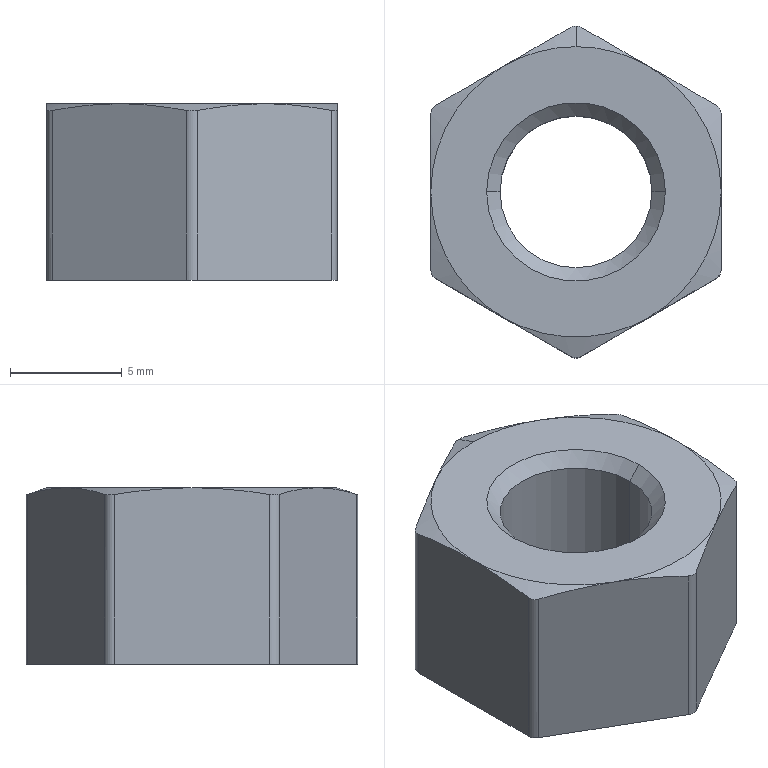Part | STEP file | 921270336 | 1 solid | 27 faces | box 13 x 14.856 x 7.9 mm | volume 859.126 mm3 | cone 11 | cylinder 8 | plane 8 | commonest cylinder face diameters 1 x6 6.8 x2
STEP:
#1=CARTESIAN_POINT('',(3.4,0.,7.3));
#2=VERTEX_POINT('',#1);
#3=CARTESIAN_POINT('',(-3.4,0.,7.3));
#4=VERTEX_POINT('',#3);
#5=CARTESIAN_POINT('',(0.,0.,7.3));
#6=DIRECTION('',(0.,0.,-1.));
#7=DIRECTION('',(-1.,0.,0.));
#8=AXIS2_PLACEMENT_3D('',#5,#6,#7);
#9=CIRCLE('',#8,3.4);
#10=EDGE_CURVE('',#2,#4,#9,.T.);
#11=ORIENTED_EDGE('',*,*,#10,.F.);
#12=CARTESIAN_POINT('',(3.4,0.,0.6));
#13=VERTEX_POINT('',#12);
#14=CARTESIAN_POINT('',(3.4,0.,7.9));
#15=DIRECTION('',(0.,0.,-1.));
#16=VECTOR('',#15,1000.);
#17=LINE('',#14,#16);
#18=EDGE_CURVE('',#2,#13,#17,.T.);
#19=ORIENTED_EDGE('',*,*,#18,.T.);
#20=CARTESIAN_POINT('',(-3.4,0.,0.6));
#21=VERTEX_POINT('',#20);
#22=CARTESIAN_POINT('',(0.,0.,0.6));
#23=DIRECTION('',(0.,0.,1.));
#24=DIRECTION('',(-1.,0.,0.));
#25=AXIS2_PLACEMENT_3D('',#22,#23,#24);
#26=CIRCLE('',#25,3.4);
#27=EDGE_CURVE('',#21,#13,#26,.T.);
#28=ORIENTED_EDGE('',*,*,#27,.F.);
#29=CARTESIAN_POINT('',(-3.4,0.,7.9));
#30=DIRECTION('',(0.,0.,-1.));
#31=VECTOR('',#30,1000.);
#32=LINE('',#29,#31);
#33=EDGE_CURVE('',#4,#21,#32,.T.);
#34=ORIENTED_EDGE('',*,*,#33,.F.);
#35=EDGE_LOOP('',(#11,#19,#28,#34));
#36=FACE_OUTER_BOUND('',#35,.T.);
#37=CARTESIAN_POINT('',(0.,0.,7.9));
#38=DIRECTION('',(0.,0.,-1.));
#39=DIRECTION('',(-1.,0.,0.));
#40=AXIS2_PLACEMENT_3D('',#37,#38,#39);
#41=CYLINDRICAL_SURFACE('',#40,3.4);
#42=ADVANCED_FACE('',(#36),#41,.F.);
#43=ORIENTED_EDGE('',*,*,#10,.T.);
#44=CARTESIAN_POINT('',(-4.,0.,7.9));
#45=VERTEX_POINT('',#44);
#46=CARTESIAN_POINT('',(-4.,0.,7.9));
#47=DIRECTION('',(-0.7071,0.,0.7071));
#48=VECTOR('',#47,1000.);
#49=LINE('',#46,#48);
#50=EDGE_CURVE('',#4,#45,#49,.T.);
#51=ORIENTED_EDGE('',*,*,#50,.T.);
#52=CARTESIAN_POINT('',(4.,0.,7.9));
#53=VERTEX_POINT('',#52);
#54=CARTESIAN_POINT('',(0.,0.,7.9));
#55=DIRECTION('',(0.,0.,-1.));
#56=DIRECTION('',(1.,0.,0.));
#57=AXIS2_PLACEMENT_3D('',#54,#55,#56);
#58=CIRCLE('',#57,4.);
#59=EDGE_CURVE('',#53,#45,#58,.T.);
#60=ORIENTED_EDGE('',*,*,#59,.F.);
#61=CARTESIAN_POINT('',(4.,0.,7.9));
#62=DIRECTION('',(0.7071,0.,0.7071));
#63=VECTOR('',#62,1000.);
#64=LINE('',#61,#63);
#65=EDGE_CURVE('',#2,#53,#64,.T.);
#66=ORIENTED_EDGE('',*,*,#65,.F.);
#67=EDGE_LOOP('',(#43,#51,#60,#66));
#68=FACE_OUTER_BOUND('',#67,.T.);
#69=CARTESIAN_POINT('',(0.,0.,7.9));
#70=DIRECTION('',(0.,0.,1.));
#71=DIRECTION('',(1.,0.,0.));
#72=AXIS2_PLACEMENT_3D('',#69,#70,#71);
#73=CONICAL_SURFACE('',#72,4.,0.7854);
#74=ADVANCED_FACE('',(#68),#73,.F.);
#75=ORIENTED_EDGE('',*,*,#27,.T.);
#76=CARTESIAN_POINT('',(4.,0.,0.));
#77=VERTEX_POINT('',#76);
#78=CARTESIAN_POINT('',(4.,0.,0.));
#79=DIRECTION('',(0.7071,0.,-0.7071));
#80=VECTOR('',#79,1000.);
#81=LINE('',#78,#80);
#82=EDGE_CURVE('',#13,#77,#81,.T.);
#83=ORIENTED_EDGE('',*,*,#82,.T.);
#84=CARTESIAN_POINT('',(-4.,0.,0.));
#85=VERTEX_POINT('',#84);
#86=CARTESIAN_POINT('',(0.,0.,0.));
#87=DIRECTION('',(0.,0.,1.));
#88=DIRECTION('',(-1.,0.,0.));
#89=AXIS2_PLACEMENT_3D('',#86,#87,#88);
#90=CIRCLE('',#89,4.);
#91=EDGE_CURVE('',#85,#77,#90,.T.);
#92=ORIENTED_EDGE('',*,*,#91,.F.);
#93=CARTESIAN_POINT('',(-4.,0.,0.));
#94=DIRECTION('',(-0.7071,0.,-0.7071));
#95=VECTOR('',#94,1000.);
#96=LINE('',#93,#95);
#97=EDGE_CURVE('',#21,#85,#96,.T.);
#98=ORIENTED_EDGE('',*,*,#97,.F.);
#99=EDGE_LOOP('',(#75,#83,#92,#98));
#100=FACE_OUTER_BOUND('',#99,.T.);
#101=CARTESIAN_POINT('',(0.,0.,0.));
#102=DIRECTION('',(0.,0.,-1.));
#103=DIRECTION('',(-1.,0.,0.));
#104=AXIS2_PLACEMENT_3D('',#101,#102,#103);
#105=CONICAL_SURFACE('',#104,4.,0.7854);
#106=ADVANCED_FACE('',(#100),#105,.F.);
#107=CARTESIAN_POINT('',(0.,6.5,7.9));
#108=VERTEX_POINT('',#107);
#109=CARTESIAN_POINT('',(-3.25,5.629,7.9));
#110=VERTEX_POINT('',#109);
#111=CARTESIAN_POINT('',(0.,0.,7.9));
#112=DIRECTION('',(0.,0.,1.));
#113=DIRECTION('',(0.,1.,0.));
#114=AXIS2_PLACEMENT_3D('',#111,#112,#113);
#115=CIRCLE('',#114,6.5);
#116=EDGE_CURVE('',#108,#110,#115,.T.);
#117=ORIENTED_EDGE('',*,*,#116,.F.);
#118=CARTESIAN_POINT('',(0.,7.428,7.58));
#119=VERTEX_POINT('',#118);
#120=CARTESIAN_POINT('',(0.,7.434,7.578));
#121=DIRECTION('',(0.,0.9455,-0.3256));
#122=VECTOR('',#121,1000.);
#123=LINE('',#120,#122);
#124=EDGE_CURVE('',#108,#119,#123,.T.);
#125=ORIENTED_EDGE('',*,*,#124,.T.);
#126=CARTESIAN_POINT('',(-0.25,7.361,7.602));
#127=VERTEX_POINT('',#126);
#128=CARTESIAN_POINT('',(-0.25,7.361,7.602));
#129=CARTESIAN_POINT('',(-0.1743,7.405,7.588));
#130=CARTESIAN_POINT('',(-0.08732,7.428,7.58));
#131=CARTESIAN_POINT('',(0.,7.428,7.58));
#132=B_SPLINE_CURVE_WITH_KNOTS('',3,(#128,#129,#130,#131),.UNSPECIFIED.,.F.,.F.,(4,4),(0.,0.0002619),.UNSPECIFIED.);
#133=EDGE_CURVE('',#127,#119,#132,.T.);
#134=ORIENTED_EDGE('',*,*,#133,.F.);
#135=CARTESIAN_POINT('',(-0.25,7.361,7.602));
#136=CARTESIAN_POINT('',(-1.244,6.788,7.788));
#137=CARTESIAN_POINT('',(-2.243,6.211,7.9));
#138=CARTESIAN_POINT('',(-3.25,5.629,7.9));
#139=B_SPLINE_CURVE_WITH_KNOTS('',3,(#135,#136,#137,#138),.UNSPECIFIED.,.F.,.F.,(4,4),(0.,0.003477),.UNSPECIFIED.);
#140=EDGE_CURVE('',#127,#110,#139,.T.);
#141=ORIENTED_EDGE('',*,*,#140,.T.);
#142=EDGE_LOOP('',(#117,#125,#134,#141));
#143=FACE_OUTER_BOUND('',#142,.T.);
#144=CARTESIAN_POINT('',(0.,0.,7.578));
#145=DIRECTION('',(0.,0.,-1.));
#146=DIRECTION('',(0.,1.,0.));
#147=AXIS2_PLACEMENT_3D('',#144,#145,#146);
#148=CONICAL_SURFACE('',#147,7.434,1.239);
#149=ADVANCED_FACE('',(#143),#148,.T.);
#150=ORIENTED_EDGE('',*,*,#18,.F.);
#151=CARTESIAN_POINT('',(0.,0.,7.3));
#152=DIRECTION('',(0.,0.,-1.));
#153=DIRECTION('',(-1.,0.,0.));
#154=AXIS2_PLACEMENT_3D('',#151,#152,#153);
#155=CIRCLE('',#154,3.4);
#156=EDGE_CURVE('',#4,#2,#155,.T.);
#157=ORIENTED_EDGE('',*,*,#156,.F.);
#158=ORIENTED_EDGE('',*,*,#33,.T.);
#159=CARTESIAN_POINT('',(0.,0.,0.6));
#160=DIRECTION('',(0.,0.,1.));
#161=DIRECTION('',(-1.,0.,0.));
#162=AXIS2_PLACEMENT_3D('',#159,#160,#161);
#163=CIRCLE('',#162,3.4);
#164=EDGE_CURVE('',#13,#21,#163,.T.);
#165=ORIENTED_EDGE('',*,*,#164,.F.);
#166=EDGE_LOOP('',(#150,#157,#158,#165));
#167=FACE_OUTER_BOUND('',#166,.T.);
#168=CARTESIAN_POINT('',(0.,0.,7.9));
#169=DIRECTION('',(0.,0.,-1.));
#170=DIRECTION('',(-1.,0.,0.));
#171=AXIS2_PLACEMENT_3D('',#168,#169,#170);
#172=CYLINDRICAL_SURFACE('',#171,3.4);
#173=ADVANCED_FACE('',(#167),#172,.F.);
#174=ORIENTED_EDGE('',*,*,#50,.F.);
#175=ORIENTED_EDGE('',*,*,#156,.T.);
#176=ORIENTED_EDGE('',*,*,#65,.T.);
#177=CARTESIAN_POINT('',(0.,0.,7.9));
#178=DIRECTION('',(0.,0.,-1.));
#179=DIRECTION('',(1.,0.,0.));
#180=AXIS2_PLACEMENT_3D('',#177,#178,#179);
#181=CIRCLE('',#180,4.);
#182=EDGE_CURVE('',#45,#53,#181,.T.);
#183=ORIENTED_EDGE('',*,*,#182,.F.);
#184=EDGE_LOOP('',(#174,#175,#176,#183));
#185=FACE_OUTER_BOUND('',#184,.T.);
#186=CARTESIAN_POINT('',(0.,0.,7.9));
#187=DIRECTION('',(0.,0.,1.));
#188=DIRECTION('',(1.,0.,0.));
#189=AXIS2_PLACEMENT_3D('',#186,#187,#188);
#190=CONICAL_SURFACE('',#189,4.,0.7854);
#191=ADVANCED_FACE('',(#185),#190,.F.);
#192=ORIENTED_EDGE('',*,*,#82,.F.);
#193=ORIENTED_EDGE('',*,*,#164,.T.);
#194=ORIENTED_EDGE('',*,*,#97,.T.);
#195=CARTESIAN_POINT('',(0.,0.,0.));
#196=DIRECTION('',(0.,0.,1.));
#197=DIRECTION('',(-1.,0.,0.));
#198=AXIS2_PLACEMENT_3D('',#195,#196,#197);
#199=CIRCLE('',#198,4.);
#200=EDGE_CURVE('',#77,#85,#199,.T.);
#201=ORIENTED_EDGE('',*,*,#200,.F.);
#202=EDGE_LOOP('',(#192,#193,#194,#201));
#203=FACE_OUTER_BOUND('',#202,.T.);
#204=CARTESIAN_POINT('',(0.,0.,0.));
#205=DIRECTION('',(0.,0.,-1.));
#206=DIRECTION('',(-1.,0.,0.));
#207=AXIS2_PLACEMENT_3D('',#204,#205,#206);
#208=CONICAL_SURFACE('',#207,4.,0.7854);
#209=ADVANCED_FACE('',(#203),#208,.F.);
#210=ORIENTED_EDGE('',*,*,#59,.T.);
#211=ORIENTED_EDGE('',*,*,#182,.T.);
#212=EDGE_LOOP('',(#210,#211));
#213=FACE_BOUND('',#212,.T.);
#214=CARTESIAN_POINT('',(-6.5,0.,7.9));
#215=VERTEX_POINT('',#214);
#216=CARTESIAN_POINT('',(-3.25,-5.629,7.9));
#217=VERTEX_POINT('',#216);
#218=CARTESIAN_POINT('',(0.,0.,7.9));
#219=DIRECTION('',(0.,0.,1.));
#220=DIRECTION('',(0.,1.,0.));
#221=AXIS2_PLACEMENT_3D('',#218,#219,#220);
#222=CIRCLE('',#221,6.5);
#223=EDGE_CURVE('',#215,#217,#222,.T.);
#224=ORIENTED_EDGE('',*,*,#223,.T.);
#225=CARTESIAN_POINT('',(3.25,-5.629,7.9));
#226=VERTEX_POINT('',#225);
#227=CARTESIAN_POINT('',(0.,0.,7.9));
#228=DIRECTION('',(0.,0.,1.));
#229=DIRECTION('',(0.,1.,0.));
#230=AXIS2_PLACEMENT_3D('',#227,#228,#229);
#231=CIRCLE('',#230,6.5);
#232=EDGE_CURVE('',#217,#226,#231,.T.);
#233=ORIENTED_EDGE('',*,*,#232,.T.);
#234=CARTESIAN_POINT('',(6.5,0.,7.9));
#235=VERTEX_POINT('',#234);
#236=CARTESIAN_POINT('',(0.,0.,7.9));
#237=DIRECTION('',(0.,0.,1.));
#238=DIRECTION('',(0.,1.,0.));
#239=AXIS2_PLACEMENT_3D('',#236,#237,#238);
#240=CIRCLE('',#239,6.5);
#241=EDGE_CURVE('',#226,#235,#240,.T.);
#242=ORIENTED_EDGE('',*,*,#241,.T.);
#243=CARTESIAN_POINT('',(3.25,5.629,7.9));
#244=VERTEX_POINT('',#243);
#245=CARTESIAN_POINT('',(0.,0.,7.9));
#246=DIRECTION('',(0.,0.,1.));
#247=DIRECTION('',(0.,1.,0.));
#248=AXIS2_PLACEMENT_3D('',#245,#246,#247);
#249=CIRCLE('',#248,6.5);
#250=EDGE_CURVE('',#235,#244,#249,.T.);
#251=ORIENTED_EDGE('',*,*,#250,.T.);
#252=CARTESIAN_POINT('',(0.,0.,7.9));
#253=DIRECTION('',(0.,0.,1.));
#254=DIRECTION('',(0.,1.,0.));
#255=AXIS2_PLACEMENT_3D('',#252,#253,#254);
#256=CIRCLE('',#255,6.5);
#257=EDGE_CURVE('',#244,#108,#256,.T.);
#258=ORIENTED_EDGE('',*,*,#257,.T.);
#259=ORIENTED_EDGE('',*,*,#116,.T.);
#260=CARTESIAN_POINT('',(0.,0.,7.9));
#261=DIRECTION('',(0.,0.,1.));
#262=DIRECTION('',(0.,1.,0.));
#263=AXIS2_PLACEMENT_3D('',#260,#261,#262);
#264=CIRCLE('',#263,6.5);
#265=EDGE_CURVE('',#110,#215,#264,.T.);
#266=ORIENTED_EDGE('',*,*,#265,.T.);
#267=EDGE_LOOP('',(#224,#233,#242,#251,#258,#259,#266));
#268=FACE_OUTER_BOUND('',#267,.T.);
#269=CARTESIAN_POINT('',(0.,7.506,7.9));
#270=DIRECTION('',(0.,0.,1.));
#271=DIRECTION('',(1.,0.,0.));
#272=AXIS2_PLACEMENT_3D('',#269,#270,#271);
#273=PLANE('',#272);
#274=ADVANCED_FACE('',(#213,#268),#273,.T.);
#275=CARTESIAN_POINT('',(-6.25,3.897,0.));
#276=VERTEX_POINT('',#275);
#277=CARTESIAN_POINT('',(-6.5,3.464,0.));
#278=VERTEX_POINT('',#277);
#279=CARTESIAN_POINT('',(-6.,3.464,0.));
#280=DIRECTION('',(0.,0.,1.));
#281=DIRECTION('',(-1.,0.,0.));
#282=AXIS2_PLACEMENT_3D('',#279,#280,#281);
#283=CIRCLE('',#282,0.5);
#284=EDGE_CURVE('',#276,#278,#283,.T.);
#285=ORIENTED_EDGE('',*,*,#284,.F.);
#286=CARTESIAN_POINT('',(-0.25,7.361,0.));
#287=VERTEX_POINT('',#286);
#288=CARTESIAN_POINT('',(-0.25,7.361,0.));
#289=DIRECTION('',(-0.866,-0.5,0.));
#290=VECTOR('',#289,1000.);
#291=LINE('',#288,#290);
#292=EDGE_CURVE('',#287,#276,#291,.T.);
#293=ORIENTED_EDGE('',*,*,#292,.F.);
#294=CARTESIAN_POINT('',(0.25,7.361,0.));
#295=VERTEX_POINT('',#294);
#296=CARTESIAN_POINT('',(0.,6.928,0.));
#297=DIRECTION('',(0.,0.,1.));
#298=DIRECTION('',(-1.,0.,0.));
#299=AXIS2_PLACEMENT_3D('',#296,#297,#298);
#300=CIRCLE('',#299,0.5);
#301=EDGE_CURVE('',#295,#287,#300,.T.);
#302=ORIENTED_EDGE('',*,*,#301,.F.);
#303=CARTESIAN_POINT('',(6.25,3.897,0.));
#304=VERTEX_POINT('',#303);
#305=CARTESIAN_POINT('',(6.25,3.897,0.));
#306=DIRECTION('',(-0.866,0.5,0.));
#307=VECTOR('',#306,1000.);
#308=LINE('',#305,#307);
#309=EDGE_CURVE('',#304,#295,#308,.T.);
#310=ORIENTED_EDGE('',*,*,#309,.F.);
#311=CARTESIAN_POINT('',(6.5,3.464,0.));
#312=VERTEX_POINT('',#311);
#313=CARTESIAN_POINT('',(6.,3.464,0.));
#314=DIRECTION('',(0.,0.,1.));
#315=DIRECTION('',(-1.,0.,0.));
#316=AXIS2_PLACEMENT_3D('',#313,#314,#315);
#317=CIRCLE('',#316,0.5);
#318=EDGE_CURVE('',#312,#304,#317,.T.);
#319=ORIENTED_EDGE('',*,*,#318,.F.);
#320=CARTESIAN_POINT('',(6.5,-3.464,0.));
#321=VERTEX_POINT('',#320);
#322=CARTESIAN_POINT('',(6.5,7.506,0.));
#323=DIRECTION('',(0.,1.,0.));
#324=VECTOR('',#323,1000.);
#325=LINE('',#322,#324);
#326=EDGE_CURVE('',#321,#312,#325,.T.);
#327=ORIENTED_EDGE('',*,*,#326,.F.);
#328=CARTESIAN_POINT('',(6.25,-3.897,0.));
#329=VERTEX_POINT('',#328);
#330=CARTESIAN_POINT('',(6.,-3.464,0.));
#331=DIRECTION('',(0.,0.,1.));
#332=DIRECTION('',(-1.,0.,0.));
#333=AXIS2_PLACEMENT_3D('',#330,#331,#332);
#334=CIRCLE('',#333,0.5);
#335=EDGE_CURVE('',#329,#321,#334,.T.);
#336=ORIENTED_EDGE('',*,*,#335,.F.);
#337=CARTESIAN_POINT('',(0.25,-7.361,0.));
#338=VERTEX_POINT('',#337);
#339=CARTESIAN_POINT('',(0.25,-7.361,0.));
#340=DIRECTION('',(0.866,0.5,0.));
#341=VECTOR('',#340,1000.);
#342=LINE('',#339,#341);
#343=EDGE_CURVE('',#338,#329,#342,.T.);
#344=ORIENTED_EDGE('',*,*,#343,.F.);
#345=CARTESIAN_POINT('',(-0.25,-7.361,0.));
#346=VERTEX_POINT('',#345);
#347=CARTESIAN_POINT('',(0.,-6.928,0.));
#348=DIRECTION('',(0.,0.,1.));
#349=DIRECTION('',(-1.,0.,0.));
#350=AXIS2_PLACEMENT_3D('',#347,#348,#349);
#351=CIRCLE('',#350,0.5);
#352=EDGE_CURVE('',#346,#338,#351,.T.);
#353=ORIENTED_EDGE('',*,*,#352,.F.);
#354=CARTESIAN_POINT('',(-6.25,-3.897,0.));
#355=VERTEX_POINT('',#354);
#356=CARTESIAN_POINT('',(-6.25,-3.897,0.));
#357=DIRECTION('',(0.866,-0.5,0.));
#358=VECTOR('',#357,1000.);
#359=LINE('',#356,#358);
#360=EDGE_CURVE('',#355,#346,#359,.T.);
#361=ORIENTED_EDGE('',*,*,#360,.F.);
#362=CARTESIAN_POINT('',(-6.5,-3.464,0.));
#363=VERTEX_POINT('',#362);
#364=CARTESIAN_POINT('',(-6.,-3.464,0.));
#365=DIRECTION('',(0.,0.,1.));
#366=DIRECTION('',(-1.,0.,0.));
#367=AXIS2_PLACEMENT_3D('',#364,#365,#366);
#368=CIRCLE('',#367,0.5);
#369=EDGE_CURVE('',#363,#355,#368,.T.);
#370=ORIENTED_EDGE('',*,*,#369,.F.);
#371=CARTESIAN_POINT('',(-6.5,7.506,0.));
#372=DIRECTION('',(0.,-1.,0.));
#373=VECTOR('',#372,1000.);
#374=LINE('',#371,#373);
#375=EDGE_CURVE('',#278,#363,#374,.T.);
#376=ORIENTED_EDGE('',*,*,#375,.F.);
#377=EDGE_LOOP('',(#285,#293,#302,#310,#319,#327,#336,#344,#353,#361,#370,#376));
#378=FACE_OUTER_BOUND('',#377,.T.);
#379=ORIENTED_EDGE('',*,*,#91,.T.);
#380=ORIENTED_EDGE('',*,*,#200,.T.);
#381=EDGE_LOOP('',(#379,#380));
#382=FACE_BOUND('',#381,.T.);
#383=CARTESIAN_POINT('',(0.,7.506,0.));
#384=DIRECTION('',(0.,0.,1.));
#385=DIRECTION('',(1.,0.,0.));
#386=AXIS2_PLACEMENT_3D('',#383,#384,#385);
#387=PLANE('',#386);
#388=ADVANCED_FACE('',(#378,#382),#387,.F.);
#389=CARTESIAN_POINT('',(0.25,-7.361,7.602));
#390=VERTEX_POINT('',#389);
#391=CARTESIAN_POINT('',(0.25,-7.361,7.602));
#392=CARTESIAN_POINT('',(1.244,-6.788,7.788));
#393=CARTESIAN_POINT('',(2.243,-6.211,7.9));
#394=CARTESIAN_POINT('',(3.25,-5.629,7.9));
#395=B_SPLINE_CURVE_WITH_KNOTS('',3,(#391,#392,#393,#394),.UNSPECIFIED.,.F.,.F.,(4,4),(0.,0.003477),.UNSPECIFIED.);
#396=EDGE_CURVE('',#390,#226,#395,.T.);
#397=ORIENTED_EDGE('',*,*,#396,.T.);
#398=ORIENTED_EDGE('',*,*,#232,.F.);
#399=CARTESIAN_POINT('',(-0.25,-7.361,7.602));
#400=VERTEX_POINT('',#399);
#401=CARTESIAN_POINT('',(-3.25,-5.629,7.9));
#402=CARTESIAN_POINT('',(-2.243,-6.211,7.9));
#403=CARTESIAN_POINT('',(-1.244,-6.788,7.788));
#404=CARTESIAN_POINT('',(-0.25,-7.361,7.602));
#405=B_SPLINE_CURVE_WITH_KNOTS('',3,(#401,#402,#403,#404),.UNSPECIFIED.,.F.,.F.,(4,4),(0.,0.003477),.UNSPECIFIED.);
#406=EDGE_CURVE('',#217,#400,#405,.T.);
#407=ORIENTED_EDGE('',*,*,#406,.T.);
#408=CARTESIAN_POINT('',(0.25,-7.361,7.602));
#409=CARTESIAN_POINT('',(0.1744,-7.405,7.588));
#410=CARTESIAN_POINT('',(0.0875,-7.428,7.58));
#411=CARTESIAN_POINT('',(-0.08695,-7.428,7.58));
#412=CARTESIAN_POINT('',(-0.1744,-7.405,7.588));
#413=CARTESIAN_POINT('',(-0.25,-7.361,7.602));
#414=B_SPLINE_CURVE_WITH_KNOTS('',3,(#408,#409,#410,#411,#412,#413),.UNSPECIFIED.,.F.,.F.,(4,2,4),(0.,0.0002616,0.0005231),.UNSPECIFIED.);
#415=EDGE_CURVE('',#390,#400,#414,.T.);
#416=ORIENTED_EDGE('',*,*,#415,.F.);
#417=EDGE_LOOP('',(#397,#398,#407,#416));
#418=FACE_OUTER_BOUND('',#417,.T.);
#419=CARTESIAN_POINT('',(0.,0.,7.578));
#420=DIRECTION('',(0.,0.,-1.));
#421=DIRECTION('',(0.,1.,0.));
#422=AXIS2_PLACEMENT_3D('',#419,#420,#421);
#423=CONICAL_SURFACE('',#422,7.434,1.239);
#424=ADVANCED_FACE('',(#418),#423,.T.);
#425=CARTESIAN_POINT('',(-6.25,-3.897,7.602));
#426=VERTEX_POINT('',#425);
#427=CARTESIAN_POINT('',(-6.25,-3.897,7.602));
#428=CARTESIAN_POINT('',(-5.256,-4.471,7.788));
#429=CARTESIAN_POINT('',(-4.257,-5.048,7.9));
#430=CARTESIAN_POINT('',(-3.25,-5.629,7.9));
#431=B_SPLINE_CURVE_WITH_KNOTS('',3,(#427,#428,#429,#430),.UNSPECIFIED.,.F.,.F.,(4,4),(0.,0.003477),.UNSPECIFIED.);
#432=EDGE_CURVE('',#426,#217,#431,.T.);
#433=ORIENTED_EDGE('',*,*,#432,.T.);
#434=ORIENTED_EDGE('',*,*,#223,.F.);
#435=CARTESIAN_POINT('',(-6.5,-3.464,7.602));
#436=VERTEX_POINT('',#435);
#437=CARTESIAN_POINT('',(-6.5,0.,7.9));
#438=CARTESIAN_POINT('',(-6.5,-1.163,7.9));
#439=CARTESIAN_POINT('',(-6.5,-2.317,7.788));
#440=CARTESIAN_POINT('',(-6.5,-3.464,7.602));
#441=B_SPLINE_CURVE_WITH_KNOTS('',3,(#437,#438,#439,#440),.UNSPECIFIED.,.F.,.F.,(4,4),(0.,0.003477),.UNSPECIFIED.);
#442=EDGE_CURVE('',#215,#436,#441,.T.);
#443=ORIENTED_EDGE('',*,*,#442,.T.);
#444=CARTESIAN_POINT('',(-6.25,-3.897,7.602));
#445=CARTESIAN_POINT('',(-6.326,-3.853,7.588));
#446=CARTESIAN_POINT('',(-6.389,-3.79,7.58));
#447=CARTESIAN_POINT('',(-6.477,-3.639,7.58));
#448=CARTESIAN_POINT('',(-6.5,-3.551,7.588));
#449=CARTESIAN_POINT('',(-6.5,-3.464,7.602));
#450=B_SPLINE_CURVE_WITH_KNOTS('',3,(#444,#445,#446,#447,#448,#449),.UNSPECIFIED.,.F.,.F.,(4,2,4),(0.,0.0002616,0.0005231),.UNSPECIFIED.);
#451=EDGE_CURVE('',#426,#436,#450,.T.);
#452=ORIENTED_EDGE('',*,*,#451,.F.);
#453=EDGE_LOOP('',(#433,#434,#443,#452));
#454=FACE_OUTER_BOUND('',#453,.T.);
#455=CARTESIAN_POINT('',(0.,0.,7.578));
#456=DIRECTION('',(0.,0.,-1.));
#457=DIRECTION('',(0.,1.,0.));
#458=AXIS2_PLACEMENT_3D('',#455,#456,#457);
#459=CONICAL_SURFACE('',#458,7.434,1.239);
#460=ADVANCED_FACE('',(#454),#459,.T.);
#461=CARTESIAN_POINT('',(-6.5,3.464,7.602));
#462=VERTEX_POINT('',#461);
#463=CARTESIAN_POINT('',(-6.5,3.464,7.602));
#464=CARTESIAN_POINT('',(-6.5,2.317,7.788));
#465=CARTESIAN_POINT('',(-6.5,1.163,7.9));
#466=CARTESIAN_POINT('',(-6.5,0.,7.9));
#467=B_SPLINE_CURVE_WITH_KNOTS('',3,(#463,#464,#465,#466),.UNSPECIFIED.,.F.,.F.,(4,4),(0.,0.003477),.UNSPECIFIED.);
#468=EDGE_CURVE('',#462,#215,#467,.T.);
#469=ORIENTED_EDGE('',*,*,#468,.T.);
#470=ORIENTED_EDGE('',*,*,#265,.F.);
#471=CARTESIAN_POINT('',(-6.25,3.897,7.602));
#472=VERTEX_POINT('',#471);
#473=CARTESIAN_POINT('',(-3.25,5.629,7.9));
#474=CARTESIAN_POINT('',(-4.257,5.048,7.9));
#475=CARTESIAN_POINT('',(-5.256,4.471,7.788));
#476=CARTESIAN_POINT('',(-6.25,3.897,7.602));
#477=B_SPLINE_CURVE_WITH_KNOTS('',3,(#473,#474,#475,#476),.UNSPECIFIED.,.F.,.F.,(4,4),(0.,0.003477),.UNSPECIFIED.);
#478=EDGE_CURVE('',#110,#472,#477,.T.);
#479=ORIENTED_EDGE('',*,*,#478,.T.);
#480=CARTESIAN_POINT('',(-6.5,3.464,7.602));
#481=CARTESIAN_POINT('',(-6.5,3.551,7.588));
#482=CARTESIAN_POINT('',(-6.477,3.638,7.58));
#483=CARTESIAN_POINT('',(-6.39,3.789,7.58));
#484=CARTESIAN_POINT('',(-6.326,3.853,7.588));
#485=CARTESIAN_POINT('',(-6.25,3.897,7.602));
#486=B_SPLINE_CURVE_WITH_KNOTS('',3,(#480,#481,#482,#483,#484,#485),.UNSPECIFIED.,.F.,.F.,(4,2,4),(0.,0.0002616,0.0005231),.UNSPECIFIED.);
#487=EDGE_CURVE('',#462,#472,#486,.T.);
#488=ORIENTED_EDGE('',*,*,#487,.F.);
#489=EDGE_LOOP('',(#469,#470,#479,#488));
#490=FACE_OUTER_BOUND('',#489,.T.);
#491=CARTESIAN_POINT('',(0.,0.,7.578));
#492=DIRECTION('',(0.,0.,-1.));
#493=DIRECTION('',(0.,1.,0.));
#494=AXIS2_PLACEMENT_3D('',#491,#492,#493);
#495=CONICAL_SURFACE('',#494,7.434,1.239);
#496=ADVANCED_FACE('',(#490),#495,.T.);
#497=ORIENTED_EDGE('',*,*,#124,.F.);
#498=ORIENTED_EDGE('',*,*,#257,.F.);
#499=CARTESIAN_POINT('',(0.25,7.361,7.602));
#500=VERTEX_POINT('',#499);
#501=CARTESIAN_POINT('',(3.25,5.629,7.9));
#502=CARTESIAN_POINT('',(2.243,6.211,7.9));
#503=CARTESIAN_POINT('',(1.244,6.788,7.788));
#504=CARTESIAN_POINT('',(0.25,7.361,7.602));
#505=B_SPLINE_CURVE_WITH_KNOTS('',3,(#501,#502,#503,#504),.UNSPECIFIED.,.F.,.F.,(4,4),(0.,0.003477),.UNSPECIFIED.);
#506=EDGE_CURVE('',#244,#500,#505,.T.);
#507=ORIENTED_EDGE('',*,*,#506,.T.);
#508=CARTESIAN_POINT('',(0.,7.428,7.58));
#509=CARTESIAN_POINT('',(0.08714,7.428,7.58));
#510=CARTESIAN_POINT('',(0.1745,7.405,7.588));
#511=CARTESIAN_POINT('',(0.25,7.361,7.602));
#512=B_SPLINE_CURVE_WITH_KNOTS('',3,(#508,#509,#510,#511),.UNSPECIFIED.,.F.,.F.,(4,4),(0.0002619,0.0005231),.UNSPECIFIED.);
#513=EDGE_CURVE('',#119,#500,#512,.T.);
#514=ORIENTED_EDGE('',*,*,#513,.F.);
#515=EDGE_LOOP('',(#497,#498,#507,#514));
#516=FACE_OUTER_BOUND('',#515,.T.);
#517=CARTESIAN_POINT('',(0.,0.,7.578));
#518=DIRECTION('',(0.,0.,-1.));
#519=DIRECTION('',(0.,1.,0.));
#520=AXIS2_PLACEMENT_3D('',#517,#518,#519);
#521=CONICAL_SURFACE('',#520,7.434,1.239);
#522=ADVANCED_FACE('',(#516),#521,.T.);
#523=CARTESIAN_POINT('',(6.25,3.897,7.602));
#524=VERTEX_POINT('',#523);
#525=CARTESIAN_POINT('',(6.25,3.897,7.602));
#526=CARTESIAN_POINT('',(5.256,4.471,7.788));
#527=CARTESIAN_POINT('',(4.257,5.048,7.9));
#528=CARTESIAN_POINT('',(3.25,5.629,7.9));
#529=B_SPLINE_CURVE_WITH_KNOTS('',3,(#525,#526,#527,#528),.UNSPECIFIED.,.F.,.F.,(4,4),(0.,0.003477),.UNSPECIFIED.);
#530=EDGE_CURVE('',#524,#244,#529,.T.);
#531=ORIENTED_EDGE('',*,*,#530,.T.);
#532=ORIENTED_EDGE('',*,*,#250,.F.);
#533=CARTESIAN_POINT('',(6.5,3.464,7.602));
#534=VERTEX_POINT('',#533);
#535=CARTESIAN_POINT('',(6.5,0.,7.9));
#536=CARTESIAN_POINT('',(6.5,1.163,7.9));
#537=CARTESIAN_POINT('',(6.5,2.317,7.788));
#538=CARTESIAN_POINT('',(6.5,3.464,7.602));
#539=B_SPLINE_CURVE_WITH_KNOTS('',3,(#535,#536,#537,#538),.UNSPECIFIED.,.F.,.F.,(4,4),(0.,0.003477),.UNSPECIFIED.);
#540=EDGE_CURVE('',#235,#534,#539,.T.);
#541=ORIENTED_EDGE('',*,*,#540,.T.);
#542=CARTESIAN_POINT('',(6.25,3.897,7.602));
#543=CARTESIAN_POINT('',(6.326,3.853,7.588));
#544=CARTESIAN_POINT('',(6.389,3.79,7.58));
#545=CARTESIAN_POINT('',(6.477,3.639,7.58));
#546=CARTESIAN_POINT('',(6.5,3.551,7.588));
#547=CARTESIAN_POINT('',(6.5,3.464,7.602));
#548=B_SPLINE_CURVE_WITH_KNOTS('',3,(#542,#543,#544,#545,#546,#547),.UNSPECIFIED.,.F.,.F.,(4,2,4),(0.,0.0002616,0.0005231),.UNSPECIFIED.);
#549=EDGE_CURVE('',#524,#534,#548,.T.);
#550=ORIENTED_EDGE('',*,*,#549,.F.);
#551=EDGE_LOOP('',(#531,#532,#541,#550));
#552=FACE_OUTER_BOUND('',#551,.T.);
#553=CARTESIAN_POINT('',(0.,0.,7.578));
#554=DIRECTION('',(0.,0.,-1.));
#555=DIRECTION('',(0.,1.,0.));
#556=AXIS2_PLACEMENT_3D('',#553,#554,#555);
#557=CONICAL_SURFACE('',#556,7.434,1.239);
#558=ADVANCED_FACE('',(#552),#557,.T.);
#559=CARTESIAN_POINT('',(6.5,-3.464,7.602));
#560=VERTEX_POINT('',#559);
#561=CARTESIAN_POINT('',(6.5,-3.464,7.602));
#562=CARTESIAN_POINT('',(6.5,-2.317,7.788));
#563=CARTESIAN_POINT('',(6.5,-1.163,7.9));
#564=CARTESIAN_POINT('',(6.5,0.,7.9));
#565=B_SPLINE_CURVE_WITH_KNOTS('',3,(#561,#562,#563,#564),.UNSPECIFIED.,.F.,.F.,(4,4),(0.,0.003477),.UNSPECIFIED.);
#566=EDGE_CURVE('',#560,#235,#565,.T.);
#567=ORIENTED_EDGE('',*,*,#566,.T.);
#568=ORIENTED_EDGE('',*,*,#241,.F.);
#569=CARTESIAN_POINT('',(6.25,-3.897,7.602));
#570=VERTEX_POINT('',#569);
#571=CARTESIAN_POINT('',(3.25,-5.629,7.9));
#572=CARTESIAN_POINT('',(4.257,-5.048,7.9));
#573=CARTESIAN_POINT('',(5.256,-4.471,7.788));
#574=CARTESIAN_POINT('',(6.25,-3.897,7.602));
#575=B_SPLINE_CURVE_WITH_KNOTS('',3,(#571,#572,#573,#574),.UNSPECIFIED.,.F.,.F.,(4,4),(0.,0.003477),.UNSPECIFIED.);
#576=EDGE_CURVE('',#226,#570,#575,.T.);
#577=ORIENTED_EDGE('',*,*,#576,.T.);
#578=CARTESIAN_POINT('',(6.5,-3.464,7.602));
#579=CARTESIAN_POINT('',(6.5,-3.551,7.588));
#580=CARTESIAN_POINT('',(6.477,-3.638,7.58));
#581=CARTESIAN_POINT('',(6.39,-3.789,7.58));
#582=CARTESIAN_POINT('',(6.326,-3.853,7.588));
#583=CARTESIAN_POINT('',(6.25,-3.897,7.602));
#584=B_SPLINE_CURVE_WITH_KNOTS('',3,(#578,#579,#580,#581,#582,#583),.UNSPECIFIED.,.F.,.F.,(4,2,4),(0.,0.0002616,0.0005231),.UNSPECIFIED.);
#585=EDGE_CURVE('',#560,#570,#584,.T.);
#586=ORIENTED_EDGE('',*,*,#585,.F.);
#587=EDGE_LOOP('',(#567,#568,#577,#586));
#588=FACE_OUTER_BOUND('',#587,.T.);
#589=CARTESIAN_POINT('',(0.,0.,7.578));
#590=DIRECTION('',(0.,0.,-1.));
#591=DIRECTION('',(0.,1.,0.));
#592=AXIS2_PLACEMENT_3D('',#589,#590,#591);
#593=CONICAL_SURFACE('',#592,7.434,1.239);
#594=ADVANCED_FACE('',(#588),#593,.T.);
#595=CARTESIAN_POINT('',(-6.5,3.464,7.9));
#596=DIRECTION('',(0.,0.,1.));
#597=VECTOR('',#596,1000.);
#598=LINE('',#595,#597);
#599=EDGE_CURVE('',#278,#462,#598,.T.);
#600=ORIENTED_EDGE('',*,*,#599,.F.);
#601=ORIENTED_EDGE('',*,*,#375,.T.);
#602=CARTESIAN_POINT('',(-6.5,-3.464,7.9));
#603=DIRECTION('',(0.,0.,-1.));
#604=VECTOR('',#603,1000.);
#605=LINE('',#602,#604);
#606=EDGE_CURVE('',#436,#363,#605,.T.);
#607=ORIENTED_EDGE('',*,*,#606,.F.);
#608=ORIENTED_EDGE('',*,*,#442,.F.);
#609=ORIENTED_EDGE('',*,*,#468,.F.);
#610=EDGE_LOOP('',(#600,#601,#607,#608,#609));
#611=FACE_OUTER_BOUND('',#610,.T.);
#612=CARTESIAN_POINT('',(-6.5,3.753,7.9));
#613=DIRECTION('',(1.,0.,0.));
#614=DIRECTION('',(0.,1.,0.));
#615=AXIS2_PLACEMENT_3D('',#612,#613,#614);
#616=PLANE('',#615);
#617=ADVANCED_FACE('',(#611),#616,.F.);
#618=CARTESIAN_POINT('',(-6.25,3.897,7.9));
#619=DIRECTION('',(0.,0.,-1.));
#620=VECTOR('',#619,1000.);
#621=LINE('',#618,#620);
#622=EDGE_CURVE('',#472,#276,#621,.T.);
#623=ORIENTED_EDGE('',*,*,#622,.F.);
#624=ORIENTED_EDGE('',*,*,#478,.F.);
#625=ORIENTED_EDGE('',*,*,#140,.F.);
#626=CARTESIAN_POINT('',(-0.25,7.361,7.9));
#627=DIRECTION('',(0.,0.,1.));
#628=VECTOR('',#627,1000.);
#629=LINE('',#626,#628);
#630=EDGE_CURVE('',#287,#127,#629,.T.);
#631=ORIENTED_EDGE('',*,*,#630,.F.);
#632=ORIENTED_EDGE('',*,*,#292,.T.);
#633=EDGE_LOOP('',(#623,#624,#625,#631,#632));
#634=FACE_OUTER_BOUND('',#633,.T.);
#635=CARTESIAN_POINT('',(0.,7.506,7.9));
#636=DIRECTION('',(0.5,-0.866,0.));
#637=DIRECTION('',(0.866,0.5,0.));
#638=AXIS2_PLACEMENT_3D('',#635,#636,#637);
#639=PLANE('',#638);
#640=ADVANCED_FACE('',(#634),#639,.F.);
#641=CARTESIAN_POINT('',(6.25,3.897,7.9));
#642=DIRECTION('',(0.,0.,1.));
#643=VECTOR('',#642,1000.);
#644=LINE('',#641,#643);
#645=EDGE_CURVE('',#304,#524,#644,.T.);
#646=ORIENTED_EDGE('',*,*,#645,.F.);
#647=ORIENTED_EDGE('',*,*,#309,.T.);
#648=CARTESIAN_POINT('',(0.25,7.361,7.9));
#649=DIRECTION('',(0.,0.,-1.));
#650=VECTOR('',#649,1000.);
#651=LINE('',#648,#650);
#652=EDGE_CURVE('',#500,#295,#651,.T.);
#653=ORIENTED_EDGE('',*,*,#652,.F.);
#654=ORIENTED_EDGE('',*,*,#506,.F.);
#655=ORIENTED_EDGE('',*,*,#530,.F.);
#656=EDGE_LOOP('',(#646,#647,#653,#654,#655));
#657=FACE_OUTER_BOUND('',#656,.T.);
#658=CARTESIAN_POINT('',(6.5,3.753,7.9));
#659=DIRECTION('',(-0.5,-0.866,0.));
#660=DIRECTION('',(0.866,-0.5,0.));
#661=AXIS2_PLACEMENT_3D('',#658,#659,#660);
#662=PLANE('',#661);
#663=ADVANCED_FACE('',(#657),#662,.F.);
#664=CARTESIAN_POINT('',(6.5,-3.464,7.9));
#665=DIRECTION('',(0.,0.,1.));
#666=VECTOR('',#665,1000.);
#667=LINE('',#664,#666);
#668=EDGE_CURVE('',#321,#560,#667,.T.);
#669=ORIENTED_EDGE('',*,*,#668,.F.);
#670=ORIENTED_EDGE('',*,*,#326,.T.);
#671=CARTESIAN_POINT('',(6.5,3.464,7.9));
#672=DIRECTION('',(0.,0.,-1.));
#673=VECTOR('',#672,1000.);
#674=LINE('',#671,#673);
#675=EDGE_CURVE('',#534,#312,#674,.T.);
#676=ORIENTED_EDGE('',*,*,#675,.F.);
#677=ORIENTED_EDGE('',*,*,#540,.F.);
#678=ORIENTED_EDGE('',*,*,#566,.F.);
#679=EDGE_LOOP('',(#669,#670,#676,#677,#678));
#680=FACE_OUTER_BOUND('',#679,.T.);
#681=CARTESIAN_POINT('',(6.5,-3.753,7.9));
#682=DIRECTION('',(-1.,0.,0.));
#683=DIRECTION('',(0.,-1.,0.));
#684=AXIS2_PLACEMENT_3D('',#681,#682,#683);
#685=PLANE('',#684);
#686=ADVANCED_FACE('',(#680),#685,.F.);
#687=CARTESIAN_POINT('',(0.25,-7.361,7.9));
#688=DIRECTION('',(0.,0.,1.));
#689=VECTOR('',#688,1000.);
#690=LINE('',#687,#689);
#691=EDGE_CURVE('',#338,#390,#690,.T.);
#692=ORIENTED_EDGE('',*,*,#691,.F.);
#693=ORIENTED_EDGE('',*,*,#343,.T.);
#694=CARTESIAN_POINT('',(6.25,-3.897,7.9));
#695=DIRECTION('',(0.,0.,-1.));
#696=VECTOR('',#695,1000.);
#697=LINE('',#694,#696);
#698=EDGE_CURVE('',#570,#329,#697,.T.);
#699=ORIENTED_EDGE('',*,*,#698,.F.);
#700=ORIENTED_EDGE('',*,*,#576,.F.);
#701=ORIENTED_EDGE('',*,*,#396,.F.);
#702=EDGE_LOOP('',(#692,#693,#699,#700,#701));
#703=FACE_OUTER_BOUND('',#702,.T.);
#704=CARTESIAN_POINT('',(0.,-7.506,7.9));
#705=DIRECTION('',(-0.5,0.866,0.));
#706=DIRECTION('',(-0.866,-0.5,0.));
#707=AXIS2_PLACEMENT_3D('',#704,#705,#706);
#708=PLANE('',#707);
#709=ADVANCED_FACE('',(#703),#708,.F.);
#710=CARTESIAN_POINT('',(-6.25,-3.897,7.9));
#711=DIRECTION('',(0.,0.,1.));
#712=VECTOR('',#711,1000.);
#713=LINE('',#710,#712);
#714=EDGE_CURVE('',#355,#426,#713,.T.);
#715=ORIENTED_EDGE('',*,*,#714,.F.);
#716=ORIENTED_EDGE('',*,*,#360,.T.);
#717=CARTESIAN_POINT('',(-0.25,-7.361,7.9));
#718=DIRECTION('',(0.,0.,-1.));
#719=VECTOR('',#718,1000.);
#720=LINE('',#717,#719);
#721=EDGE_CURVE('',#400,#346,#720,.T.);
#722=ORIENTED_EDGE('',*,*,#721,.F.);
#723=ORIENTED_EDGE('',*,*,#406,.F.);
#724=ORIENTED_EDGE('',*,*,#432,.F.);
#725=EDGE_LOOP('',(#715,#716,#722,#723,#724));
#726=FACE_OUTER_BOUND('',#725,.T.);
#727=CARTESIAN_POINT('',(-6.5,-3.753,7.9));
#728=DIRECTION('',(0.5,0.866,0.));
#729=DIRECTION('',(-0.866,0.5,0.));
#730=AXIS2_PLACEMENT_3D('',#727,#728,#729);
#731=PLANE('',#730);
#732=ADVANCED_FACE('',(#726),#731,.F.);
#733=ORIENTED_EDGE('',*,*,#284,.T.);
#734=ORIENTED_EDGE('',*,*,#599,.T.);
#735=ORIENTED_EDGE('',*,*,#487,.T.);
#736=ORIENTED_EDGE('',*,*,#622,.T.);
#737=EDGE_LOOP('',(#733,#734,#735,#736));
#738=FACE_OUTER_BOUND('',#737,.T.);
#739=CARTESIAN_POINT('',(-6.,3.464,7.9));
#740=DIRECTION('',(0.,0.,-1.));
#741=DIRECTION('',(-1.,0.,0.));
#742=AXIS2_PLACEMENT_3D('',#739,#740,#741);
#743=CYLINDRICAL_SURFACE('',#742,0.5);
#744=ADVANCED_FACE('',(#738),#743,.T.);
#745=ORIENTED_EDGE('',*,*,#369,.T.);
#746=ORIENTED_EDGE('',*,*,#714,.T.);
#747=ORIENTED_EDGE('',*,*,#451,.T.);
#748=ORIENTED_EDGE('',*,*,#606,.T.);
#749=EDGE_LOOP('',(#745,#746,#747,#748));
#750=FACE_OUTER_BOUND('',#749,.T.);
#751=CARTESIAN_POINT('',(-6.,-3.464,7.9));
#752=DIRECTION('',(0.,0.,-1.));
#753=DIRECTION('',(-1.,0.,0.));
#754=AXIS2_PLACEMENT_3D('',#751,#752,#753);
#755=CYLINDRICAL_SURFACE('',#754,0.5);
#756=ADVANCED_FACE('',(#750),#755,.T.);
#757=ORIENTED_EDGE('',*,*,#301,.T.);
#758=ORIENTED_EDGE('',*,*,#630,.T.);
#759=ORIENTED_EDGE('',*,*,#133,.T.);
#760=ORIENTED_EDGE('',*,*,#513,.T.);
#761=ORIENTED_EDGE('',*,*,#652,.T.);
#762=EDGE_LOOP('',(#757,#758,#759,#760,#761));
#763=FACE_OUTER_BOUND('',#762,.T.);
#764=CARTESIAN_POINT('',(0.,6.928,7.9));
#765=DIRECTION('',(0.,0.,-1.));
#766=DIRECTION('',(-1.,0.,0.));
#767=AXIS2_PLACEMENT_3D('',#764,#765,#766);
#768=CYLINDRICAL_SURFACE('',#767,0.5);
#769=ADVANCED_FACE('',(#763),#768,.T.);
#770=ORIENTED_EDGE('',*,*,#318,.T.);
#771=ORIENTED_EDGE('',*,*,#645,.T.);
#772=ORIENTED_EDGE('',*,*,#549,.T.);
#773=ORIENTED_EDGE('',*,*,#675,.T.);
#774=EDGE_LOOP('',(#770,#771,#772,#773));
#775=FACE_OUTER_BOUND('',#774,.T.);
#776=CARTESIAN_POINT('',(6.,3.464,7.9));
#777=DIRECTION('',(0.,0.,-1.));
#778=DIRECTION('',(-1.,0.,0.));
#779=AXIS2_PLACEMENT_3D('',#776,#777,#778);
#780=CYLINDRICAL_SURFACE('',#779,0.5);
#781=ADVANCED_FACE('',(#775),#780,.T.);
#782=ORIENTED_EDGE('',*,*,#335,.T.);
#783=ORIENTED_EDGE('',*,*,#668,.T.);
#784=ORIENTED_EDGE('',*,*,#585,.T.);
#785=ORIENTED_EDGE('',*,*,#698,.T.);
#786=EDGE_LOOP('',(#782,#783,#784,#785));
#787=FACE_OUTER_BOUND('',#786,.T.);
#788=CARTESIAN_POINT('',(6.,-3.464,7.9));
#789=DIRECTION('',(0.,0.,-1.));
#790=DIRECTION('',(-1.,0.,0.));
#791=AXIS2_PLACEMENT_3D('',#788,#789,#790);
#792=CYLINDRICAL_SURFACE('',#791,0.5);
#793=ADVANCED_FACE('',(#787),#792,.T.);
#794=ORIENTED_EDGE('',*,*,#352,.T.);
#795=ORIENTED_EDGE('',*,*,#691,.T.);
#796=ORIENTED_EDGE('',*,*,#415,.T.);
#797=ORIENTED_EDGE('',*,*,#721,.T.);
#798=EDGE_LOOP('',(#794,#795,#796,#797));
#799=FACE_OUTER_BOUND('',#798,.T.);
#800=CARTESIAN_POINT('',(0.,-6.928,7.9));
#801=DIRECTION('',(0.,0.,-1.));
#802=DIRECTION('',(-1.,0.,0.));
#803=AXIS2_PLACEMENT_3D('',#800,#801,#802);
#804=CYLINDRICAL_SURFACE('',#803,0.5);
#805=ADVANCED_FACE('',(#799),#804,.T.);
#806=CLOSED_SHELL('',(#42,#74,#106,#149,#173,#191,#209,#274,#388,#424,#460,#496,#522,#558,#594,#617,#640,#663,#686,#709,#732,#744,#756,#769,#781,#793,#805));
#807=MANIFOLD_SOLID_BREP('',#806);
#808=CARTESIAN_POINT('',(0.,0.,0.));
#809=DIRECTION('',(0.,0.,1.));
#810=DIRECTION('',(1.,0.,0.));
#811=AXIS2_PLACEMENT_3D('',#808,#809,#810);
#812=(LENGTH_UNIT()NAMED_UNIT(*)SI_UNIT(.MILLI.,.METRE.));
#813=UNCERTAINTY_MEASURE_WITH_UNIT(LENGTH_MEASURE(0.00001),#812,'','');
#814=(NAMED_UNIT(*)PLANE_ANGLE_UNIT()SI_UNIT($,.RADIAN.));
#815=(NAMED_UNIT(*)SI_UNIT($,.STERADIAN.)SOLID_ANGLE_UNIT());
#816=(GEOMETRIC_REPRESENTATION_CONTEXT(3)GLOBAL_UNCERTAINTY_ASSIGNED_CONTEXT((#813))GLOBAL_UNIT_ASSIGNED_CONTEXT((#812,#814,#815))REPRESENTATION_CONTEXT('',''));
#817=ADVANCED_BREP_SHAPE_REPRESENTATION('',(#807,#811),#816);